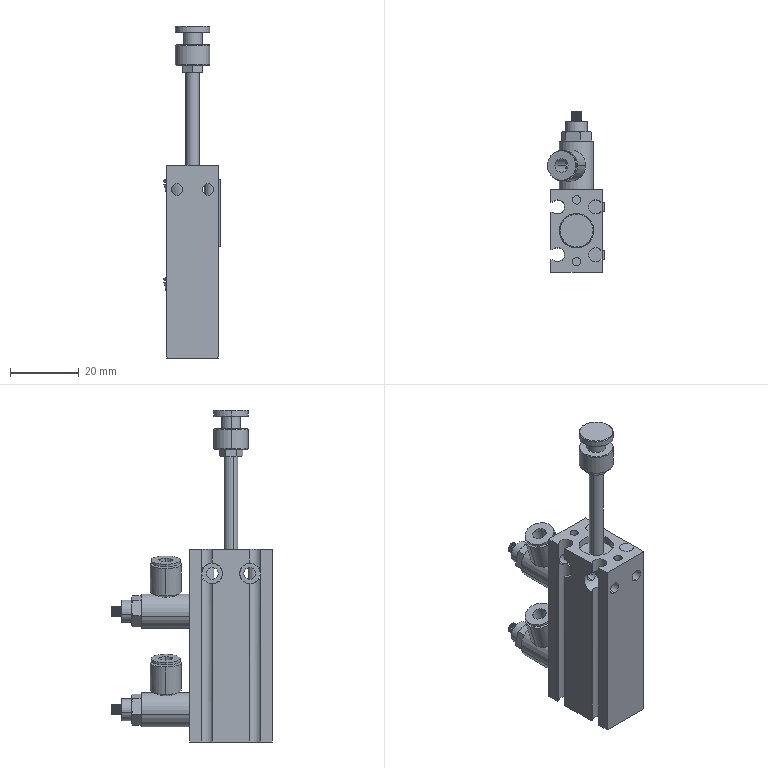Part | SolidWorks | 8 solids | 407 faces | box 16.622 x 46.7 x 96.543 mm | volume 20146 mm3 | plane 211 | cylinder 124 | cone 68 | spline 4 | commonest cylinder face diameters 10 x16 3.4 x12 6 x12 4 x10 2.459 x8 4.1 x8